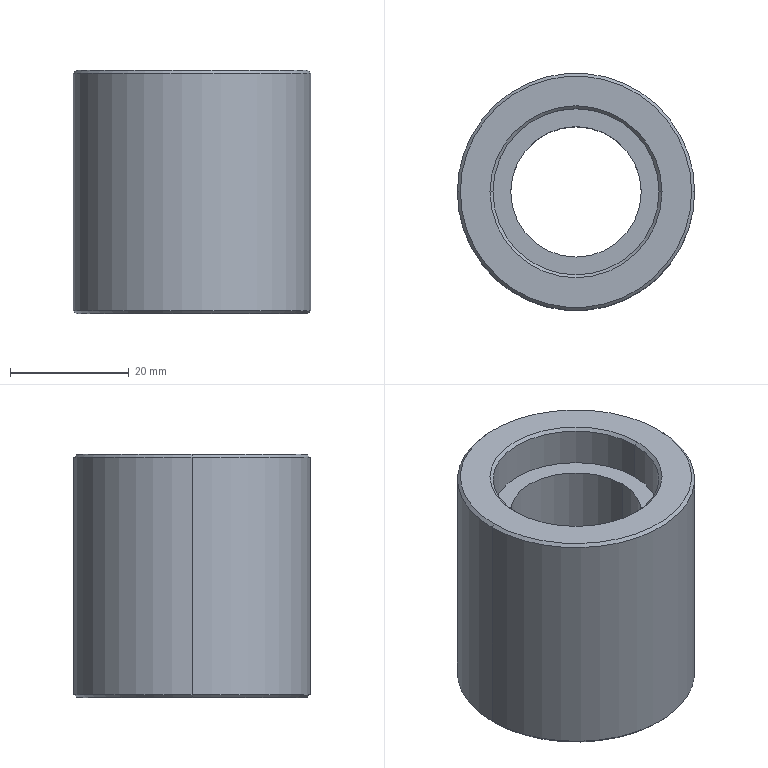Part | SolidWorks | features Chamfer 1, Extrusion 1, ICE 1, MirrorPattern 1 | 1 solid | 20 faces | box 40 x 40 x 41 mm | volume 32585 mm3 | cone 8 | cylinder 8 | plane 4 | commonest cylinder face diameters 28 x4 22 x2 40 x2
STEP:
#1=CARTESIAN_POINT('',(14.,0.,-20.));
#2=VERTEX_POINT('',#1);
#3=CARTESIAN_POINT('',(-14.,0.,-20.));
#4=VERTEX_POINT('',#3);
#5=CARTESIAN_POINT('',(0.,0.,-20.));
#6=DIRECTION('',(0.,0.,-1.));
#7=DIRECTION('',(1.,0.,0.));
#8=AXIS2_PLACEMENT_3D('',#5,#6,#7);
#9=CIRCLE('',#8,14.);
#10=EDGE_CURVE('',#2,#4,#9,.T.);
#11=ORIENTED_EDGE('',*,*,#10,.F.);
#12=CARTESIAN_POINT('',(14.5,0.,-20.5));
#13=VERTEX_POINT('',#12);
#14=CARTESIAN_POINT('',(14.5,0.,-20.5));
#15=DIRECTION('',(0.7071,0.,-0.7071));
#16=VECTOR('',#15,1000.);
#17=LINE('',#14,#16);
#18=EDGE_CURVE('',#2,#13,#17,.T.);
#19=ORIENTED_EDGE('',*,*,#18,.T.);
#20=CARTESIAN_POINT('',(-14.5,0.,-20.5));
#21=VERTEX_POINT('',#20);
#22=CARTESIAN_POINT('',(0.,0.,-20.5));
#23=DIRECTION('',(0.,0.,1.));
#24=DIRECTION('',(1.,0.,0.));
#25=AXIS2_PLACEMENT_3D('',#22,#23,#24);
#26=CIRCLE('',#25,14.5);
#27=EDGE_CURVE('',#21,#13,#26,.T.);
#28=ORIENTED_EDGE('',*,*,#27,.F.);
#29=CARTESIAN_POINT('',(-14.5,0.,-20.5));
#30=DIRECTION('',(-0.7071,0.,-0.7071));
#31=VECTOR('',#30,1000.);
#32=LINE('',#29,#31);
#33=EDGE_CURVE('',#4,#21,#32,.T.);
#34=ORIENTED_EDGE('',*,*,#33,.F.);
#35=EDGE_LOOP('',(#11,#19,#28,#34));
#36=FACE_OUTER_BOUND('',#35,.T.);
#37=CARTESIAN_POINT('',(0.,0.,-20.5));
#38=DIRECTION('',(0.,0.,-1.));
#39=DIRECTION('',(-1.,0.,0.));
#40=AXIS2_PLACEMENT_3D('',#37,#38,#39);
#41=CONICAL_SURFACE('',#40,14.5,0.7854);
#42=ADVANCED_FACE('',(#36),#41,.F.);
#43=CARTESIAN_POINT('',(-14.,0.,20.));
#44=VERTEX_POINT('',#43);
#45=CARTESIAN_POINT('',(14.,0.,20.));
#46=VERTEX_POINT('',#45);
#47=CARTESIAN_POINT('',(0.,0.,20.));
#48=DIRECTION('',(0.,0.,1.));
#49=DIRECTION('',(1.,0.,0.));
#50=AXIS2_PLACEMENT_3D('',#47,#48,#49);
#51=CIRCLE('',#50,14.);
#52=EDGE_CURVE('',#44,#46,#51,.T.);
#53=ORIENTED_EDGE('',*,*,#52,.F.);
#54=CARTESIAN_POINT('',(-14.5,0.,20.5));
#55=VERTEX_POINT('',#54);
#56=CARTESIAN_POINT('',(-14.,0.,20.));
#57=DIRECTION('',(-0.7071,0.,0.7071));
#58=VECTOR('',#57,1000.);
#59=LINE('',#56,#58);
#60=EDGE_CURVE('',#44,#55,#59,.T.);
#61=ORIENTED_EDGE('',*,*,#60,.T.);
#62=CARTESIAN_POINT('',(14.5,0.,20.5));
#63=VERTEX_POINT('',#62);
#64=CARTESIAN_POINT('',(0.,0.,20.5));
#65=DIRECTION('',(0.,0.,-1.));
#66=DIRECTION('',(1.,0.,0.));
#67=AXIS2_PLACEMENT_3D('',#64,#65,#66);
#68=CIRCLE('',#67,14.5);
#69=EDGE_CURVE('',#63,#55,#68,.T.);
#70=ORIENTED_EDGE('',*,*,#69,.F.);
#71=CARTESIAN_POINT('',(14.,0.,20.));
#72=DIRECTION('',(0.7071,0.,0.7071));
#73=VECTOR('',#72,1000.);
#74=LINE('',#71,#73);
#75=EDGE_CURVE('',#46,#63,#74,.T.);
#76=ORIENTED_EDGE('',*,*,#75,.F.);
#77=EDGE_LOOP('',(#53,#61,#70,#76));
#78=FACE_OUTER_BOUND('',#77,.T.);
#79=CARTESIAN_POINT('',(0.,0.,20.));
#80=DIRECTION('',(0.,0.,1.));
#81=DIRECTION('',(1.,0.,0.));
#82=AXIS2_PLACEMENT_3D('',#79,#80,#81);
#83=CONICAL_SURFACE('',#82,14.,0.7854);
#84=ADVANCED_FACE('',(#78),#83,.F.);
#85=CARTESIAN_POINT('',(-19.5,0.,-20.5));
#86=VERTEX_POINT('',#85);
#87=CARTESIAN_POINT('',(19.5,0.,-20.5));
#88=VERTEX_POINT('',#87);
#89=CARTESIAN_POINT('',(0.,0.,-20.5));
#90=DIRECTION('',(0.,0.,-1.));
#91=DIRECTION('',(1.,0.,0.));
#92=AXIS2_PLACEMENT_3D('',#89,#90,#91);
#93=CIRCLE('',#92,19.5);
#94=EDGE_CURVE('',#86,#88,#93,.T.);
#95=ORIENTED_EDGE('',*,*,#94,.F.);
#96=CARTESIAN_POINT('',(-20.,0.,-20.));
#97=VERTEX_POINT('',#96);
#98=CARTESIAN_POINT('',(-20.,0.,-20.));
#99=DIRECTION('',(-0.7071,0.,0.7071));
#100=VECTOR('',#99,1000.);
#101=LINE('',#98,#100);
#102=EDGE_CURVE('',#86,#97,#101,.T.);
#103=ORIENTED_EDGE('',*,*,#102,.T.);
#104=CARTESIAN_POINT('',(20.,0.,-20.));
#105=VERTEX_POINT('',#104);
#106=CARTESIAN_POINT('',(0.,0.,-20.));
#107=DIRECTION('',(0.,0.,1.));
#108=DIRECTION('',(1.,0.,0.));
#109=AXIS2_PLACEMENT_3D('',#106,#107,#108);
#110=CIRCLE('',#109,20.);
#111=EDGE_CURVE('',#105,#97,#110,.T.);
#112=ORIENTED_EDGE('',*,*,#111,.F.);
#113=CARTESIAN_POINT('',(20.,0.,-20.));
#114=DIRECTION('',(0.7071,0.,0.7071));
#115=VECTOR('',#114,1000.);
#116=LINE('',#113,#115);
#117=EDGE_CURVE('',#88,#105,#116,.T.);
#118=ORIENTED_EDGE('',*,*,#117,.F.);
#119=EDGE_LOOP('',(#95,#103,#112,#118));
#120=FACE_OUTER_BOUND('',#119,.T.);
#121=CARTESIAN_POINT('',(0.,0.,-20.));
#122=DIRECTION('',(0.,0.,1.));
#123=DIRECTION('',(1.,0.,0.));
#124=AXIS2_PLACEMENT_3D('',#121,#122,#123);
#125=CONICAL_SURFACE('',#124,20.,0.7854);
#126=ADVANCED_FACE('',(#120),#125,.T.);
#127=CARTESIAN_POINT('',(19.5,0.,20.5));
#128=VERTEX_POINT('',#127);
#129=CARTESIAN_POINT('',(-19.5,0.,20.5));
#130=VERTEX_POINT('',#129);
#131=CARTESIAN_POINT('',(0.,0.,20.5));
#132=DIRECTION('',(0.,0.,1.));
#133=DIRECTION('',(1.,0.,0.));
#134=AXIS2_PLACEMENT_3D('',#131,#132,#133);
#135=CIRCLE('',#134,19.5);
#136=EDGE_CURVE('',#128,#130,#135,.T.);
#137=ORIENTED_EDGE('',*,*,#136,.F.);
#138=CARTESIAN_POINT('',(20.,0.,20.));
#139=VERTEX_POINT('',#138);
#140=CARTESIAN_POINT('',(19.5,0.,20.5));
#141=DIRECTION('',(0.7071,0.,-0.7071));
#142=VECTOR('',#141,1000.);
#143=LINE('',#140,#142);
#144=EDGE_CURVE('',#128,#139,#143,.T.);
#145=ORIENTED_EDGE('',*,*,#144,.T.);
#146=CARTESIAN_POINT('',(-20.,0.,20.));
#147=VERTEX_POINT('',#146);
#148=CARTESIAN_POINT('',(0.,0.,20.));
#149=DIRECTION('',(0.,0.,-1.));
#150=DIRECTION('',(1.,0.,0.));
#151=AXIS2_PLACEMENT_3D('',#148,#149,#150);
#152=CIRCLE('',#151,20.);
#153=EDGE_CURVE('',#147,#139,#152,.T.);
#154=ORIENTED_EDGE('',*,*,#153,.F.);
#155=CARTESIAN_POINT('',(-19.5,0.,20.5));
#156=DIRECTION('',(-0.7071,0.,-0.7071));
#157=VECTOR('',#156,1000.);
#158=LINE('',#155,#157);
#159=EDGE_CURVE('',#130,#147,#158,.T.);
#160=ORIENTED_EDGE('',*,*,#159,.F.);
#161=EDGE_LOOP('',(#137,#145,#154,#160));
#162=FACE_OUTER_BOUND('',#161,.T.);
#163=CARTESIAN_POINT('',(0.,0.,20.5));
#164=DIRECTION('',(0.,0.,-1.));
#165=DIRECTION('',(-1.,0.,0.));
#166=AXIS2_PLACEMENT_3D('',#163,#164,#165);
#167=CONICAL_SURFACE('',#166,19.5,0.7854);
#168=ADVANCED_FACE('',(#162),#167,.T.);
#169=CARTESIAN_POINT('',(-14.,0.,-13.5));
#170=VERTEX_POINT('',#169);
#171=CARTESIAN_POINT('',(14.,0.,-13.5));
#172=VERTEX_POINT('',#171);
#173=CARTESIAN_POINT('',(0.,0.,-13.5));
#174=DIRECTION('',(0.,0.,1.));
#175=DIRECTION('',(1.,0.,0.));
#176=AXIS2_PLACEMENT_3D('',#173,#174,#175);
#177=CIRCLE('',#176,14.);
#178=EDGE_CURVE('',#170,#172,#177,.T.);
#179=ORIENTED_EDGE('',*,*,#178,.T.);
#180=CARTESIAN_POINT('',(14.,0.,-13.5));
#181=DIRECTION('',(0.,0.,-1.));
#182=VECTOR('',#181,1000.);
#183=LINE('',#180,#182);
#184=EDGE_CURVE('',#172,#2,#183,.T.);
#185=ORIENTED_EDGE('',*,*,#184,.T.);
#186=ORIENTED_EDGE('',*,*,#10,.T.);
#187=CARTESIAN_POINT('',(-14.,0.,-13.5));
#188=DIRECTION('',(0.,0.,-1.));
#189=VECTOR('',#188,1000.);
#190=LINE('',#187,#189);
#191=EDGE_CURVE('',#170,#4,#190,.T.);
#192=ORIENTED_EDGE('',*,*,#191,.F.);
#193=EDGE_LOOP('',(#179,#185,#186,#192));
#194=FACE_OUTER_BOUND('',#193,.T.);
#195=CARTESIAN_POINT('',(0.,0.,-13.5));
#196=DIRECTION('',(0.,0.,-1.));
#197=DIRECTION('',(-1.,0.,0.));
#198=AXIS2_PLACEMENT_3D('',#195,#196,#197);
#199=CYLINDRICAL_SURFACE('',#198,14.);
#200=ADVANCED_FACE('',(#194),#199,.F.);
#201=CARTESIAN_POINT('',(-14.,0.,13.5));
#202=VERTEX_POINT('',#201);
#203=CARTESIAN_POINT('',(14.,0.,13.5));
#204=VERTEX_POINT('',#203);
#205=CARTESIAN_POINT('',(0.,0.,13.5));
#206=DIRECTION('',(0.,0.,1.));
#207=DIRECTION('',(1.,0.,0.));
#208=AXIS2_PLACEMENT_3D('',#205,#206,#207);
#209=CIRCLE('',#208,14.);
#210=EDGE_CURVE('',#202,#204,#209,.T.);
#211=ORIENTED_EDGE('',*,*,#210,.F.);
#212=CARTESIAN_POINT('',(-14.,0.,13.5));
#213=DIRECTION('',(0.,0.,1.));
#214=VECTOR('',#213,1000.);
#215=LINE('',#212,#214);
#216=EDGE_CURVE('',#202,#44,#215,.T.);
#217=ORIENTED_EDGE('',*,*,#216,.T.);
#218=ORIENTED_EDGE('',*,*,#52,.T.);
#219=CARTESIAN_POINT('',(14.,0.,13.5));
#220=DIRECTION('',(0.,0.,1.));
#221=VECTOR('',#220,1000.);
#222=LINE('',#219,#221);
#223=EDGE_CURVE('',#204,#46,#222,.T.);
#224=ORIENTED_EDGE('',*,*,#223,.F.);
#225=EDGE_LOOP('',(#211,#217,#218,#224));
#226=FACE_OUTER_BOUND('',#225,.T.);
#227=CARTESIAN_POINT('',(0.,0.,13.5));
#228=DIRECTION('',(0.,0.,1.));
#229=DIRECTION('',(1.,0.,0.));
#230=AXIS2_PLACEMENT_3D('',#227,#228,#229);
#231=CYLINDRICAL_SURFACE('',#230,14.);
#232=ADVANCED_FACE('',(#226),#231,.F.);
#233=ORIENTED_EDGE('',*,*,#153,.T.);
#234=CARTESIAN_POINT('',(20.,0.,20.5));
#235=DIRECTION('',(0.,0.,-1.));
#236=VECTOR('',#235,1000.);
#237=LINE('',#234,#236);
#238=EDGE_CURVE('',#139,#105,#237,.T.);
#239=ORIENTED_EDGE('',*,*,#238,.T.);
#240=ORIENTED_EDGE('',*,*,#111,.T.);
#241=CARTESIAN_POINT('',(-20.,0.,20.5));
#242=DIRECTION('',(0.,0.,-1.));
#243=VECTOR('',#242,1000.);
#244=LINE('',#241,#243);
#245=EDGE_CURVE('',#147,#97,#244,.T.);
#246=ORIENTED_EDGE('',*,*,#245,.F.);
#247=EDGE_LOOP('',(#233,#239,#240,#246));
#248=FACE_OUTER_BOUND('',#247,.T.);
#249=CARTESIAN_POINT('',(0.,0.,20.5));
#250=DIRECTION('',(0.,0.,-1.));
#251=DIRECTION('',(-1.,0.,0.));
#252=AXIS2_PLACEMENT_3D('',#249,#250,#251);
#253=CYLINDRICAL_SURFACE('',#252,20.);
#254=ADVANCED_FACE('',(#248),#253,.T.);
#255=CARTESIAN_POINT('',(-11.,0.,13.5));
#256=VERTEX_POINT('',#255);
#257=CARTESIAN_POINT('',(11.,0.,13.5));
#258=VERTEX_POINT('',#257);
#259=CARTESIAN_POINT('',(0.,0.,13.5));
#260=DIRECTION('',(0.,0.,1.));
#261=DIRECTION('',(1.,0.,0.));
#262=AXIS2_PLACEMENT_3D('',#259,#260,#261);
#263=CIRCLE('',#262,11.);
#264=EDGE_CURVE('',#256,#258,#263,.T.);
#265=ORIENTED_EDGE('',*,*,#264,.T.);
#266=CARTESIAN_POINT('',(11.,0.,-13.5));
#267=VERTEX_POINT('',#266);
#268=CARTESIAN_POINT('',(11.,0.,20.5));
#269=DIRECTION('',(0.,0.,-1.));
#270=VECTOR('',#269,1000.);
#271=LINE('',#268,#270);
#272=EDGE_CURVE('',#258,#267,#271,.T.);
#273=ORIENTED_EDGE('',*,*,#272,.T.);
#274=CARTESIAN_POINT('',(-11.,0.,-13.5));
#275=VERTEX_POINT('',#274);
#276=CARTESIAN_POINT('',(0.,0.,-13.5));
#277=DIRECTION('',(0.,0.,-1.));
#278=DIRECTION('',(-1.,0.,0.));
#279=AXIS2_PLACEMENT_3D('',#276,#277,#278);
#280=CIRCLE('',#279,11.);
#281=EDGE_CURVE('',#267,#275,#280,.T.);
#282=ORIENTED_EDGE('',*,*,#281,.T.);
#283=CARTESIAN_POINT('',(-11.,0.,20.5));
#284=DIRECTION('',(0.,0.,-1.));
#285=VECTOR('',#284,1000.);
#286=LINE('',#283,#285);
#287=EDGE_CURVE('',#256,#275,#286,.T.);
#288=ORIENTED_EDGE('',*,*,#287,.F.);
#289=EDGE_LOOP('',(#265,#273,#282,#288));
#290=FACE_OUTER_BOUND('',#289,.T.);
#291=CARTESIAN_POINT('',(0.,0.,20.5));
#292=DIRECTION('',(0.,0.,-1.));
#293=DIRECTION('',(-1.,0.,0.));
#294=AXIS2_PLACEMENT_3D('',#291,#292,#293);
#295=CYLINDRICAL_SURFACE('',#294,11.);
#296=ADVANCED_FACE('',(#290),#295,.F.);
#297=ORIENTED_EDGE('',*,*,#272,.F.);
#298=CARTESIAN_POINT('',(0.,0.,13.5));
#299=DIRECTION('',(0.,0.,1.));
#300=DIRECTION('',(1.,0.,0.));
#301=AXIS2_PLACEMENT_3D('',#298,#299,#300);
#302=CIRCLE('',#301,11.);
#303=EDGE_CURVE('',#258,#256,#302,.T.);
#304=ORIENTED_EDGE('',*,*,#303,.T.);
#305=ORIENTED_EDGE('',*,*,#287,.T.);
#306=CARTESIAN_POINT('',(0.,0.,-13.5));
#307=DIRECTION('',(0.,0.,-1.));
#308=DIRECTION('',(-1.,0.,0.));
#309=AXIS2_PLACEMENT_3D('',#306,#307,#308);
#310=CIRCLE('',#309,11.);
#311=EDGE_CURVE('',#275,#267,#310,.T.);
#312=ORIENTED_EDGE('',*,*,#311,.T.);
#313=EDGE_LOOP('',(#297,#304,#305,#312));
#314=FACE_OUTER_BOUND('',#313,.T.);
#315=CARTESIAN_POINT('',(0.,0.,20.5));
#316=DIRECTION('',(0.,0.,-1.));
#317=DIRECTION('',(-1.,0.,0.));
#318=AXIS2_PLACEMENT_3D('',#315,#316,#317);
#319=CYLINDRICAL_SURFACE('',#318,11.);
#320=ADVANCED_FACE('',(#314),#319,.F.);
#321=CARTESIAN_POINT('',(0.,0.,-20.5));
#322=DIRECTION('',(0.,0.,-1.));
#323=DIRECTION('',(1.,0.,0.));
#324=AXIS2_PLACEMENT_3D('',#321,#322,#323);
#325=CIRCLE('',#324,19.5);
#326=EDGE_CURVE('',#88,#86,#325,.T.);
#327=ORIENTED_EDGE('',*,*,#326,.T.);
#328=ORIENTED_EDGE('',*,*,#94,.T.);
#329=EDGE_LOOP('',(#327,#328));
#330=FACE_OUTER_BOUND('',#329,.T.);
#331=ORIENTED_EDGE('',*,*,#27,.T.);
#332=CARTESIAN_POINT('',(0.,0.,-20.5));
#333=DIRECTION('',(0.,0.,1.));
#334=DIRECTION('',(1.,0.,0.));
#335=AXIS2_PLACEMENT_3D('',#332,#333,#334);
#336=CIRCLE('',#335,14.5);
#337=EDGE_CURVE('',#13,#21,#336,.T.);
#338=ORIENTED_EDGE('',*,*,#337,.T.);
#339=EDGE_LOOP('',(#331,#338));
#340=FACE_BOUND('',#339,.T.);
#341=CARTESIAN_POINT('',(0.,0.,-20.5));
#342=DIRECTION('',(0.,0.,1.));
#343=DIRECTION('',(1.,0.,0.));
#344=AXIS2_PLACEMENT_3D('',#341,#342,#343);
#345=PLANE('',#344);
#346=ADVANCED_FACE('',(#330,#340),#345,.F.);
#347=CARTESIAN_POINT('',(0.,0.,20.5));
#348=DIRECTION('',(0.,0.,1.));
#349=DIRECTION('',(1.,0.,0.));
#350=AXIS2_PLACEMENT_3D('',#347,#348,#349);
#351=CIRCLE('',#350,19.5);
#352=EDGE_CURVE('',#130,#128,#351,.T.);
#353=ORIENTED_EDGE('',*,*,#352,.T.);
#354=ORIENTED_EDGE('',*,*,#136,.T.);
#355=EDGE_LOOP('',(#353,#354));
#356=FACE_OUTER_BOUND('',#355,.T.);
#357=ORIENTED_EDGE('',*,*,#69,.T.);
#358=CARTESIAN_POINT('',(0.,0.,20.5));
#359=DIRECTION('',(0.,0.,-1.));
#360=DIRECTION('',(1.,0.,0.));
#361=AXIS2_PLACEMENT_3D('',#358,#359,#360);
#362=CIRCLE('',#361,14.5);
#363=EDGE_CURVE('',#55,#63,#362,.T.);
#364=ORIENTED_EDGE('',*,*,#363,.T.);
#365=EDGE_LOOP('',(#357,#364));
#366=FACE_BOUND('',#365,.T.);
#367=CARTESIAN_POINT('',(0.,0.,20.5));
#368=DIRECTION('',(0.,0.,1.));
#369=DIRECTION('',(1.,0.,0.));
#370=AXIS2_PLACEMENT_3D('',#367,#368,#369);
#371=PLANE('',#370);
#372=ADVANCED_FACE('',(#356,#366),#371,.T.);
#373=ORIENTED_EDGE('',*,*,#238,.F.);
#374=CARTESIAN_POINT('',(0.,0.,20.));
#375=DIRECTION('',(0.,0.,-1.));
#376=DIRECTION('',(1.,0.,0.));
#377=AXIS2_PLACEMENT_3D('',#374,#375,#376);
#378=CIRCLE('',#377,20.);
#379=EDGE_CURVE('',#139,#147,#378,.T.);
#380=ORIENTED_EDGE('',*,*,#379,.T.);
#381=ORIENTED_EDGE('',*,*,#245,.T.);
#382=CARTESIAN_POINT('',(0.,0.,-20.));
#383=DIRECTION('',(0.,0.,1.));
#384=DIRECTION('',(1.,0.,0.));
#385=AXIS2_PLACEMENT_3D('',#382,#383,#384);
#386=CIRCLE('',#385,20.);
#387=EDGE_CURVE('',#97,#105,#386,.T.);
#388=ORIENTED_EDGE('',*,*,#387,.T.);
#389=EDGE_LOOP('',(#373,#380,#381,#388));
#390=FACE_OUTER_BOUND('',#389,.T.);
#391=CARTESIAN_POINT('',(0.,0.,20.5));
#392=DIRECTION('',(0.,0.,-1.));
#393=DIRECTION('',(-1.,0.,0.));
#394=AXIS2_PLACEMENT_3D('',#391,#392,#393);
#395=CYLINDRICAL_SURFACE('',#394,20.);
#396=ADVANCED_FACE('',(#390),#395,.T.);
#397=ORIENTED_EDGE('',*,*,#216,.F.);
#398=CARTESIAN_POINT('',(0.,0.,13.5));
#399=DIRECTION('',(0.,0.,1.));
#400=DIRECTION('',(1.,0.,0.));
#401=AXIS2_PLACEMENT_3D('',#398,#399,#400);
#402=CIRCLE('',#401,14.);
#403=EDGE_CURVE('',#204,#202,#402,.T.);
#404=ORIENTED_EDGE('',*,*,#403,.F.);
#405=ORIENTED_EDGE('',*,*,#223,.T.);
#406=CARTESIAN_POINT('',(0.,0.,20.));
#407=DIRECTION('',(0.,0.,1.));
#408=DIRECTION('',(1.,0.,0.));
#409=AXIS2_PLACEMENT_3D('',#406,#407,#408);
#410=CIRCLE('',#409,14.);
#411=EDGE_CURVE('',#46,#44,#410,.T.);
#412=ORIENTED_EDGE('',*,*,#411,.T.);
#413=EDGE_LOOP('',(#397,#404,#405,#412));
#414=FACE_OUTER_BOUND('',#413,.T.);
#415=CARTESIAN_POINT('',(0.,0.,13.5));
#416=DIRECTION('',(0.,0.,1.));
#417=DIRECTION('',(1.,0.,0.));
#418=AXIS2_PLACEMENT_3D('',#415,#416,#417);
#419=CYLINDRICAL_SURFACE('',#418,14.);
#420=ADVANCED_FACE('',(#414),#419,.F.);
#421=ORIENTED_EDGE('',*,*,#264,.F.);
#422=ORIENTED_EDGE('',*,*,#303,.F.);
#423=EDGE_LOOP('',(#421,#422));
#424=FACE_BOUND('',#423,.T.);
#425=ORIENTED_EDGE('',*,*,#403,.T.);
#426=ORIENTED_EDGE('',*,*,#210,.T.);
#427=EDGE_LOOP('',(#425,#426));
#428=FACE_OUTER_BOUND('',#427,.T.);
#429=CARTESIAN_POINT('',(0.,0.,13.5));
#430=DIRECTION('',(0.,0.,1.));
#431=DIRECTION('',(1.,0.,0.));
#432=AXIS2_PLACEMENT_3D('',#429,#430,#431);
#433=PLANE('',#432);
#434=ADVANCED_FACE('',(#424,#428),#433,.T.);
#435=ORIENTED_EDGE('',*,*,#184,.F.);
#436=CARTESIAN_POINT('',(0.,0.,-13.5));
#437=DIRECTION('',(0.,0.,1.));
#438=DIRECTION('',(1.,0.,0.));
#439=AXIS2_PLACEMENT_3D('',#436,#437,#438);
#440=CIRCLE('',#439,14.);
#441=EDGE_CURVE('',#172,#170,#440,.T.);
#442=ORIENTED_EDGE('',*,*,#441,.T.);
#443=ORIENTED_EDGE('',*,*,#191,.T.);
#444=CARTESIAN_POINT('',(0.,0.,-20.));
#445=DIRECTION('',(0.,0.,-1.));
#446=DIRECTION('',(1.,0.,0.));
#447=AXIS2_PLACEMENT_3D('',#444,#445,#446);
#448=CIRCLE('',#447,14.);
#449=EDGE_CURVE('',#4,#2,#448,.T.);
#450=ORIENTED_EDGE('',*,*,#449,.T.);
#451=EDGE_LOOP('',(#435,#442,#443,#450));
#452=FACE_OUTER_BOUND('',#451,.T.);
#453=CARTESIAN_POINT('',(0.,0.,-13.5));
#454=DIRECTION('',(0.,0.,-1.));
#455=DIRECTION('',(-1.,0.,0.));
#456=AXIS2_PLACEMENT_3D('',#453,#454,#455);
#457=CYLINDRICAL_SURFACE('',#456,14.);
#458=ADVANCED_FACE('',(#452),#457,.F.);
#459=ORIENTED_EDGE('',*,*,#311,.F.);
#460=ORIENTED_EDGE('',*,*,#281,.F.);
#461=EDGE_LOOP('',(#459,#460));
#462=FACE_BOUND('',#461,.T.);
#463=ORIENTED_EDGE('',*,*,#178,.F.);
#464=ORIENTED_EDGE('',*,*,#441,.F.);
#465=EDGE_LOOP('',(#463,#464));
#466=FACE_OUTER_BOUND('',#465,.T.);
#467=CARTESIAN_POINT('',(0.,0.,-13.5));
#468=DIRECTION('',(0.,0.,-1.));
#469=DIRECTION('',(1.,0.,0.));
#470=AXIS2_PLACEMENT_3D('',#467,#468,#469);
#471=PLANE('',#470);
#472=ADVANCED_FACE('',(#462,#466),#471,.T.);
#473=ORIENTED_EDGE('',*,*,#144,.F.);
#474=ORIENTED_EDGE('',*,*,#352,.F.);
#475=ORIENTED_EDGE('',*,*,#159,.T.);
#476=ORIENTED_EDGE('',*,*,#379,.F.);
#477=EDGE_LOOP('',(#473,#474,#475,#476));
#478=FACE_OUTER_BOUND('',#477,.T.);
#479=CARTESIAN_POINT('',(0.,0.,20.5));
#480=DIRECTION('',(0.,0.,-1.));
#481=DIRECTION('',(-1.,0.,0.));
#482=AXIS2_PLACEMENT_3D('',#479,#480,#481);
#483=CONICAL_SURFACE('',#482,19.5,0.7854);
#484=ADVANCED_FACE('',(#478),#483,.T.);
#485=ORIENTED_EDGE('',*,*,#102,.F.);
#486=ORIENTED_EDGE('',*,*,#326,.F.);
#487=ORIENTED_EDGE('',*,*,#117,.T.);
#488=ORIENTED_EDGE('',*,*,#387,.F.);
#489=EDGE_LOOP('',(#485,#486,#487,#488));
#490=FACE_OUTER_BOUND('',#489,.T.);
#491=CARTESIAN_POINT('',(0.,0.,-20.));
#492=DIRECTION('',(0.,0.,1.));
#493=DIRECTION('',(1.,0.,0.));
#494=AXIS2_PLACEMENT_3D('',#491,#492,#493);
#495=CONICAL_SURFACE('',#494,20.,0.7854);
#496=ADVANCED_FACE('',(#490),#495,.T.);
#497=ORIENTED_EDGE('',*,*,#60,.F.);
#498=ORIENTED_EDGE('',*,*,#411,.F.);
#499=ORIENTED_EDGE('',*,*,#75,.T.);
#500=ORIENTED_EDGE('',*,*,#363,.F.);
#501=EDGE_LOOP('',(#497,#498,#499,#500));
#502=FACE_OUTER_BOUND('',#501,.T.);
#503=CARTESIAN_POINT('',(0.,0.,20.));
#504=DIRECTION('',(0.,0.,1.));
#505=DIRECTION('',(1.,0.,0.));
#506=AXIS2_PLACEMENT_3D('',#503,#504,#505);
#507=CONICAL_SURFACE('',#506,14.,0.7854);
#508=ADVANCED_FACE('',(#502),#507,.F.);
#509=ORIENTED_EDGE('',*,*,#18,.F.);
#510=ORIENTED_EDGE('',*,*,#449,.F.);
#511=ORIENTED_EDGE('',*,*,#33,.T.);
#512=ORIENTED_EDGE('',*,*,#337,.F.);
#513=EDGE_LOOP('',(#509,#510,#511,#512));
#514=FACE_OUTER_BOUND('',#513,.T.);
#515=CARTESIAN_POINT('',(0.,0.,-20.5));
#516=DIRECTION('',(0.,0.,-1.));
#517=DIRECTION('',(-1.,0.,0.));
#518=AXIS2_PLACEMENT_3D('',#515,#516,#517);
#519=CONICAL_SURFACE('',#518,14.5,0.7854);
#520=ADVANCED_FACE('',(#514),#519,.F.);
#521=CLOSED_SHELL('',(#42,#84,#126,#168,#200,#232,#254,#296,#320,#346,#372,#396,#420,#434,#458,#472,#484,#496,#508,#520));
#522=MANIFOLD_SOLID_BREP('',#521);
#523=CARTESIAN_POINT('',(0.,0.,0.));
#524=DIRECTION('',(0.,0.,1.));
#525=DIRECTION('',(1.,0.,0.));
#526=AXIS2_PLACEMENT_3D('',#523,#524,#525);
#527=(LENGTH_UNIT()NAMED_UNIT(*)SI_UNIT(.MILLI.,.METRE.));
#528=UNCERTAINTY_MEASURE_WITH_UNIT(LENGTH_MEASURE(0.00001),#527,'','');
#529=(NAMED_UNIT(*)PLANE_ANGLE_UNIT()SI_UNIT($,.RADIAN.));
#530=(NAMED_UNIT(*)SI_UNIT($,.STERADIAN.)SOLID_ANGLE_UNIT());
#531=(GEOMETRIC_REPRESENTATION_CONTEXT(3)GLOBAL_UNCERTAINTY_ASSIGNED_CONTEXT((#528))GLOBAL_UNIT_ASSIGNED_CONTEXT((#527,#529,#530))REPRESENTATION_CONTEXT('',''));
#532=ADVANCED_BREP_SHAPE_REPRESENTATION('',(#522,#526),#531);